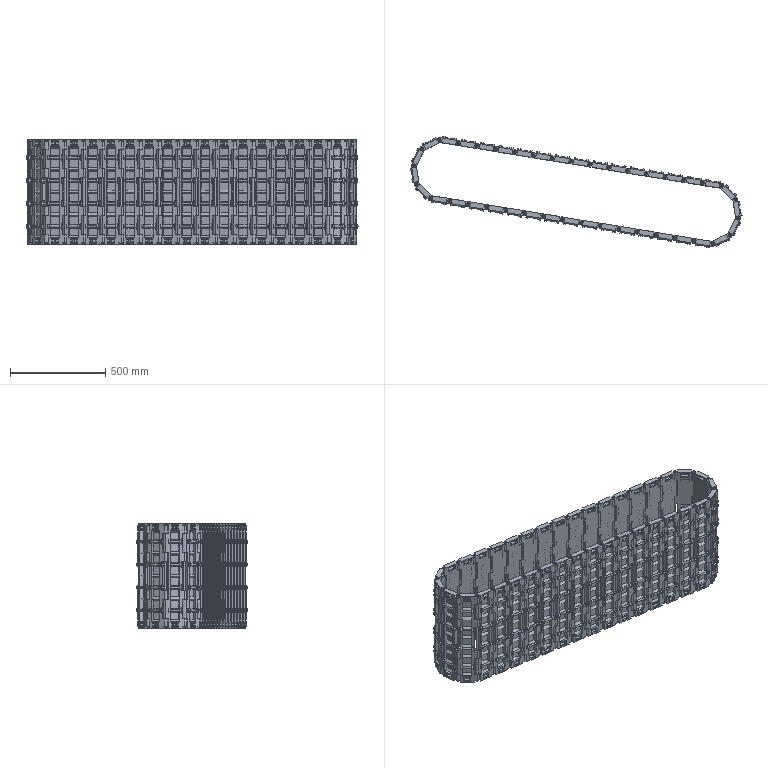Part | SolidWorks | 912 solids | 20368 faces | volume 31275893 mm3 | plane 8816 | cylinder 6992 | cone 3800 | torus 760 | commonest cylinder face diameters 3 x3648 10 x1444 8 x608 12 x608 20 x456 25 x228